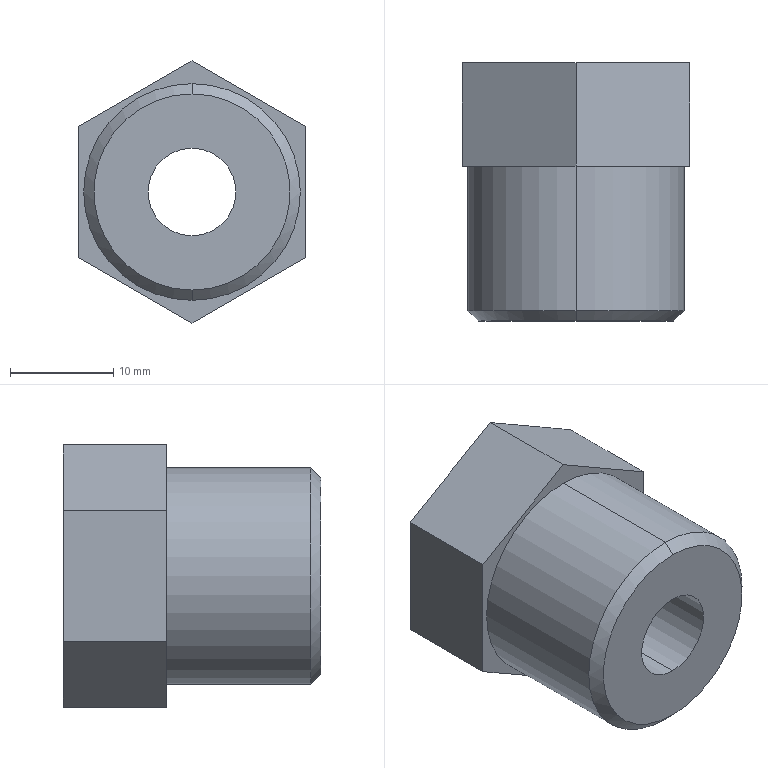Part | SolidWorks | features 3DProfileFeature 1, Chamfer 1, Extrusion 1, HoleWzd 1, ICE 1 | 1 solid | 15 faces | box 22 x 25 x 25.403 mm | volume 7936 mm3 | plane 9 | cylinder 4 | cone 2 | commonest cylinder face diameters 8.5 x2 21 x2
STEP:
#1=CARTESIAN_POINT('',(0.,0.,-4.25));
#2=VERTEX_POINT('',#1);
#3=CARTESIAN_POINT('',(0.,0.,4.25));
#4=VERTEX_POINT('',#3);
#5=CARTESIAN_POINT('',(0.,0.,0.));
#6=DIRECTION('',(0.,1.,0.));
#7=DIRECTION('',(0.,0.,1.));
#8=AXIS2_PLACEMENT_3D('',#5,#6,#7);
#9=CIRCLE('',#8,4.25);
#10=EDGE_CURVE('',#2,#4,#9,.T.);
#11=ORIENTED_EDGE('',*,*,#10,.F.);
#12=CARTESIAN_POINT('',(0.,25.,-4.25));
#13=VERTEX_POINT('',#12);
#14=CARTESIAN_POINT('',(0.,25.,-4.25));
#15=DIRECTION('',(0.,1.,0.));
#16=VECTOR('',#15,1000.);
#17=LINE('',#14,#16);
#18=EDGE_CURVE('',#2,#13,#17,.T.);
#19=ORIENTED_EDGE('',*,*,#18,.T.);
#20=CARTESIAN_POINT('',(0.,25.,4.25));
#21=VERTEX_POINT('',#20);
#22=CARTESIAN_POINT('',(0.,25.,0.));
#23=DIRECTION('',(0.,1.,0.));
#24=DIRECTION('',(0.,0.,1.));
#25=AXIS2_PLACEMENT_3D('',#22,#23,#24);
#26=CIRCLE('',#25,4.25);
#27=EDGE_CURVE('',#13,#21,#26,.T.);
#28=ORIENTED_EDGE('',*,*,#27,.T.);
#29=CARTESIAN_POINT('',(0.,25.,4.25));
#30=DIRECTION('',(0.,1.,0.));
#31=VECTOR('',#30,1000.);
#32=LINE('',#29,#31);
#33=EDGE_CURVE('',#4,#21,#32,.T.);
#34=ORIENTED_EDGE('',*,*,#33,.F.);
#35=EDGE_LOOP('',(#11,#19,#28,#34));
#36=FACE_OUTER_BOUND('',#35,.T.);
#37=CARTESIAN_POINT('',(0.,25.,0.));
#38=DIRECTION('',(0.,1.,0.));
#39=DIRECTION('',(0.,0.,1.));
#40=AXIS2_PLACEMENT_3D('',#37,#38,#39);
#41=CYLINDRICAL_SURFACE('',#40,4.25);
#42=ADVANCED_FACE('',(#36),#41,.F.);
#43=CARTESIAN_POINT('',(0.,0.,-9.5));
#44=VERTEX_POINT('',#43);
#45=CARTESIAN_POINT('',(0.,0.,9.5));
#46=VERTEX_POINT('',#45);
#47=CARTESIAN_POINT('',(0.,0.,0.));
#48=DIRECTION('',(0.,-1.,0.));
#49=DIRECTION('',(0.,0.,1.));
#50=AXIS2_PLACEMENT_3D('',#47,#48,#49);
#51=CIRCLE('',#50,9.5);
#52=EDGE_CURVE('',#44,#46,#51,.T.);
#53=ORIENTED_EDGE('',*,*,#52,.F.);
#54=CARTESIAN_POINT('',(0.,1.,-10.5));
#55=VERTEX_POINT('',#54);
#56=CARTESIAN_POINT('',(0.,0.,-9.5));
#57=DIRECTION('',(0.,0.7071,-0.7071));
#58=VECTOR('',#57,1000.);
#59=LINE('',#56,#58);
#60=EDGE_CURVE('',#44,#55,#59,.T.);
#61=ORIENTED_EDGE('',*,*,#60,.T.);
#62=CARTESIAN_POINT('',(0.,1.,10.5));
#63=VERTEX_POINT('',#62);
#64=CARTESIAN_POINT('',(0.,1.,0.));
#65=DIRECTION('',(0.,1.,0.));
#66=DIRECTION('',(0.,0.,1.));
#67=AXIS2_PLACEMENT_3D('',#64,#65,#66);
#68=CIRCLE('',#67,10.5);
#69=EDGE_CURVE('',#63,#55,#68,.T.);
#70=ORIENTED_EDGE('',*,*,#69,.F.);
#71=CARTESIAN_POINT('',(0.,0.,9.5));
#72=DIRECTION('',(0.,0.7071,0.7071));
#73=VECTOR('',#72,1000.);
#74=LINE('',#71,#73);
#75=EDGE_CURVE('',#46,#63,#74,.T.);
#76=ORIENTED_EDGE('',*,*,#75,.F.);
#77=EDGE_LOOP('',(#53,#61,#70,#76));
#78=FACE_OUTER_BOUND('',#77,.T.);
#79=CARTESIAN_POINT('',(0.,0.,0.));
#80=DIRECTION('',(0.,1.,0.));
#81=DIRECTION('',(0.,0.,1.));
#82=AXIS2_PLACEMENT_3D('',#79,#80,#81);
#83=CONICAL_SURFACE('',#82,9.5,0.7854);
#84=ADVANCED_FACE('',(#78),#83,.T.);
#85=CARTESIAN_POINT('',(0.,15.,-10.5));
#86=VERTEX_POINT('',#85);
#87=CARTESIAN_POINT('',(0.,15.,10.5));
#88=VERTEX_POINT('',#87);
#89=CARTESIAN_POINT('',(0.,15.,0.));
#90=DIRECTION('',(0.,-1.,0.));
#91=DIRECTION('',(0.,0.,1.));
#92=AXIS2_PLACEMENT_3D('',#89,#90,#91);
#93=CIRCLE('',#92,10.5);
#94=EDGE_CURVE('',#86,#88,#93,.T.);
#95=ORIENTED_EDGE('',*,*,#94,.T.);
#96=CARTESIAN_POINT('',(0.,58.942,10.5));
#97=DIRECTION('',(0.,-1.,0.));
#98=VECTOR('',#97,1000.);
#99=LINE('',#96,#98);
#100=EDGE_CURVE('',#88,#63,#99,.T.);
#101=ORIENTED_EDGE('',*,*,#100,.T.);
#102=ORIENTED_EDGE('',*,*,#69,.T.);
#103=CARTESIAN_POINT('',(0.,58.942,-10.5));
#104=DIRECTION('',(0.,-1.,0.));
#105=VECTOR('',#104,1000.);
#106=LINE('',#103,#105);
#107=EDGE_CURVE('',#86,#55,#106,.T.);
#108=ORIENTED_EDGE('',*,*,#107,.F.);
#109=EDGE_LOOP('',(#95,#101,#102,#108));
#110=FACE_OUTER_BOUND('',#109,.T.);
#111=CARTESIAN_POINT('',(0.,58.942,0.));
#112=DIRECTION('',(0.,-1.,0.));
#113=DIRECTION('',(0.,0.,-1.));
#114=AXIS2_PLACEMENT_3D('',#111,#112,#113);
#115=CYLINDRICAL_SURFACE('',#114,10.5);
#116=ADVANCED_FACE('',(#110),#115,.T.);
#117=CARTESIAN_POINT('',(0.,25.,12.702));
#118=VERTEX_POINT('',#117);
#119=CARTESIAN_POINT('',(0.,15.,12.702));
#120=VERTEX_POINT('',#119);
#121=CARTESIAN_POINT('',(0.,25.,12.702));
#122=DIRECTION('',(0.,-1.,0.));
#123=VECTOR('',#122,1000.);
#124=LINE('',#121,#123);
#125=EDGE_CURVE('',#118,#120,#124,.T.);
#126=ORIENTED_EDGE('',*,*,#125,.T.);
#127=CARTESIAN_POINT('',(11.,15.,6.351));
#128=VERTEX_POINT('',#127);
#129=CARTESIAN_POINT('',(0.,15.,12.702));
#130=DIRECTION('',(0.866,0.,-0.5));
#131=VECTOR('',#130,1000.);
#132=LINE('',#129,#131);
#133=EDGE_CURVE('',#120,#128,#132,.T.);
#134=ORIENTED_EDGE('',*,*,#133,.T.);
#135=CARTESIAN_POINT('',(11.,25.,6.351));
#136=VERTEX_POINT('',#135);
#137=CARTESIAN_POINT('',(11.,25.,6.351));
#138=DIRECTION('',(0.,-1.,0.));
#139=VECTOR('',#138,1000.);
#140=LINE('',#137,#139);
#141=EDGE_CURVE('',#136,#128,#140,.T.);
#142=ORIENTED_EDGE('',*,*,#141,.F.);
#143=CARTESIAN_POINT('',(0.,25.,12.702));
#144=DIRECTION('',(0.866,0.,-0.5));
#145=VECTOR('',#144,1000.);
#146=LINE('',#143,#145);
#147=EDGE_CURVE('',#118,#136,#146,.T.);
#148=ORIENTED_EDGE('',*,*,#147,.F.);
#149=EDGE_LOOP('',(#126,#134,#142,#148));
#150=FACE_OUTER_BOUND('',#149,.T.);
#151=CARTESIAN_POINT('',(0.,25.,12.702));
#152=DIRECTION('',(-0.5,0.,-0.866));
#153=DIRECTION('',(-0.866,0.,0.5));
#154=AXIS2_PLACEMENT_3D('',#151,#152,#153);
#155=PLANE('',#154);
#156=ADVANCED_FACE('',(#150),#155,.F.);
#157=ORIENTED_EDGE('',*,*,#141,.T.);
#158=CARTESIAN_POINT('',(11.,15.,-6.351));
#159=VERTEX_POINT('',#158);
#160=CARTESIAN_POINT('',(11.,15.,6.351));
#161=DIRECTION('',(0.,0.,-1.));
#162=VECTOR('',#161,1000.);
#163=LINE('',#160,#162);
#164=EDGE_CURVE('',#128,#159,#163,.T.);
#165=ORIENTED_EDGE('',*,*,#164,.T.);
#166=CARTESIAN_POINT('',(11.,25.,-6.351));
#167=VERTEX_POINT('',#166);
#168=CARTESIAN_POINT('',(11.,25.,-6.351));
#169=DIRECTION('',(0.,-1.,0.));
#170=VECTOR('',#169,1000.);
#171=LINE('',#168,#170);
#172=EDGE_CURVE('',#167,#159,#171,.T.);
#173=ORIENTED_EDGE('',*,*,#172,.F.);
#174=CARTESIAN_POINT('',(11.,25.,6.351));
#175=DIRECTION('',(0.,0.,-1.));
#176=VECTOR('',#175,1000.);
#177=LINE('',#174,#176);
#178=EDGE_CURVE('',#136,#167,#177,.T.);
#179=ORIENTED_EDGE('',*,*,#178,.F.);
#180=EDGE_LOOP('',(#157,#165,#173,#179));
#181=FACE_OUTER_BOUND('',#180,.T.);
#182=CARTESIAN_POINT('',(11.,25.,6.351));
#183=DIRECTION('',(-1.,0.,0.));
#184=DIRECTION('',(0.,0.,1.));
#185=AXIS2_PLACEMENT_3D('',#182,#183,#184);
#186=PLANE('',#185);
#187=ADVANCED_FACE('',(#181),#186,.F.);
#188=ORIENTED_EDGE('',*,*,#172,.T.);
#189=CARTESIAN_POINT('',(0.,15.,-12.702));
#190=VERTEX_POINT('',#189);
#191=CARTESIAN_POINT('',(11.,15.,-6.351));
#192=DIRECTION('',(-0.866,0.,-0.5));
#193=VECTOR('',#192,1000.);
#194=LINE('',#191,#193);
#195=EDGE_CURVE('',#159,#190,#194,.T.);
#196=ORIENTED_EDGE('',*,*,#195,.T.);
#197=CARTESIAN_POINT('',(0.,25.,-12.702));
#198=VERTEX_POINT('',#197);
#199=CARTESIAN_POINT('',(0.,25.,-12.702));
#200=DIRECTION('',(0.,-1.,0.));
#201=VECTOR('',#200,1000.);
#202=LINE('',#199,#201);
#203=EDGE_CURVE('',#198,#190,#202,.T.);
#204=ORIENTED_EDGE('',*,*,#203,.F.);
#205=CARTESIAN_POINT('',(11.,25.,-6.351));
#206=DIRECTION('',(-0.866,0.,-0.5));
#207=VECTOR('',#206,1000.);
#208=LINE('',#205,#207);
#209=EDGE_CURVE('',#167,#198,#208,.T.);
#210=ORIENTED_EDGE('',*,*,#209,.F.);
#211=EDGE_LOOP('',(#188,#196,#204,#210));
#212=FACE_OUTER_BOUND('',#211,.T.);
#213=CARTESIAN_POINT('',(11.,25.,-6.351));
#214=DIRECTION('',(-0.5,0.,0.866));
#215=DIRECTION('',(0.866,0.,0.5));
#216=AXIS2_PLACEMENT_3D('',#213,#214,#215);
#217=PLANE('',#216);
#218=ADVANCED_FACE('',(#212),#217,.F.);
#219=ORIENTED_EDGE('',*,*,#203,.T.);
#220=CARTESIAN_POINT('',(-11.,15.,-6.351));
#221=VERTEX_POINT('',#220);
#222=CARTESIAN_POINT('',(0.,15.,-12.702));
#223=DIRECTION('',(-0.866,0.,0.5));
#224=VECTOR('',#223,1000.);
#225=LINE('',#222,#224);
#226=EDGE_CURVE('',#190,#221,#225,.T.);
#227=ORIENTED_EDGE('',*,*,#226,.T.);
#228=CARTESIAN_POINT('',(-11.,25.,-6.351));
#229=VERTEX_POINT('',#228);
#230=CARTESIAN_POINT('',(-11.,25.,-6.351));
#231=DIRECTION('',(0.,-1.,0.));
#232=VECTOR('',#231,1000.);
#233=LINE('',#230,#232);
#234=EDGE_CURVE('',#229,#221,#233,.T.);
#235=ORIENTED_EDGE('',*,*,#234,.F.);
#236=CARTESIAN_POINT('',(0.,25.,-12.702));
#237=DIRECTION('',(-0.866,0.,0.5));
#238=VECTOR('',#237,1000.);
#239=LINE('',#236,#238);
#240=EDGE_CURVE('',#198,#229,#239,.T.);
#241=ORIENTED_EDGE('',*,*,#240,.F.);
#242=EDGE_LOOP('',(#219,#227,#235,#241));
#243=FACE_OUTER_BOUND('',#242,.T.);
#244=CARTESIAN_POINT('',(0.,25.,-12.702));
#245=DIRECTION('',(0.5,0.,0.866));
#246=DIRECTION('',(0.866,0.,-0.5));
#247=AXIS2_PLACEMENT_3D('',#244,#245,#246);
#248=PLANE('',#247);
#249=ADVANCED_FACE('',(#243),#248,.F.);
#250=ORIENTED_EDGE('',*,*,#234,.T.);
#251=CARTESIAN_POINT('',(-11.,15.,6.351));
#252=VERTEX_POINT('',#251);
#253=CARTESIAN_POINT('',(-11.,15.,-6.351));
#254=DIRECTION('',(0.,0.,1.));
#255=VECTOR('',#254,1000.);
#256=LINE('',#253,#255);
#257=EDGE_CURVE('',#221,#252,#256,.T.);
#258=ORIENTED_EDGE('',*,*,#257,.T.);
#259=CARTESIAN_POINT('',(-11.,25.,6.351));
#260=VERTEX_POINT('',#259);
#261=CARTESIAN_POINT('',(-11.,25.,6.351));
#262=DIRECTION('',(0.,-1.,0.));
#263=VECTOR('',#262,1000.);
#264=LINE('',#261,#263);
#265=EDGE_CURVE('',#260,#252,#264,.T.);
#266=ORIENTED_EDGE('',*,*,#265,.F.);
#267=CARTESIAN_POINT('',(-11.,25.,-6.351));
#268=DIRECTION('',(0.,0.,1.));
#269=VECTOR('',#268,1000.);
#270=LINE('',#267,#269);
#271=EDGE_CURVE('',#229,#260,#270,.T.);
#272=ORIENTED_EDGE('',*,*,#271,.F.);
#273=EDGE_LOOP('',(#250,#258,#266,#272));
#274=FACE_OUTER_BOUND('',#273,.T.);
#275=CARTESIAN_POINT('',(-11.,25.,-6.351));
#276=DIRECTION('',(1.,0.,0.));
#277=DIRECTION('',(0.,0.,-1.));
#278=AXIS2_PLACEMENT_3D('',#275,#276,#277);
#279=PLANE('',#278);
#280=ADVANCED_FACE('',(#274),#279,.F.);
#281=ORIENTED_EDGE('',*,*,#265,.T.);
#282=CARTESIAN_POINT('',(-11.,15.,6.351));
#283=DIRECTION('',(0.866,0.,0.5));
#284=VECTOR('',#283,1000.);
#285=LINE('',#282,#284);
#286=EDGE_CURVE('',#252,#120,#285,.T.);
#287=ORIENTED_EDGE('',*,*,#286,.T.);
#288=ORIENTED_EDGE('',*,*,#125,.F.);
#289=CARTESIAN_POINT('',(-11.,25.,6.351));
#290=DIRECTION('',(0.866,0.,0.5));
#291=VECTOR('',#290,1000.);
#292=LINE('',#289,#291);
#293=EDGE_CURVE('',#260,#118,#292,.T.);
#294=ORIENTED_EDGE('',*,*,#293,.F.);
#295=EDGE_LOOP('',(#281,#287,#288,#294));
#296=FACE_OUTER_BOUND('',#295,.T.);
#297=CARTESIAN_POINT('',(-11.,25.,6.351));
#298=DIRECTION('',(0.5,0.,-0.866));
#299=DIRECTION('',(-0.866,0.,-0.5));
#300=AXIS2_PLACEMENT_3D('',#297,#298,#299);
#301=PLANE('',#300);
#302=ADVANCED_FACE('',(#296),#301,.F.);
#303=CARTESIAN_POINT('',(0.,25.,0.));
#304=DIRECTION('',(0.,1.,0.));
#305=DIRECTION('',(0.,0.,1.));
#306=AXIS2_PLACEMENT_3D('',#303,#304,#305);
#307=CIRCLE('',#306,4.25);
#308=EDGE_CURVE('',#21,#13,#307,.T.);
#309=ORIENTED_EDGE('',*,*,#308,.F.);
#310=ORIENTED_EDGE('',*,*,#27,.F.);
#311=EDGE_LOOP('',(#309,#310));
#312=FACE_BOUND('',#311,.T.);
#313=ORIENTED_EDGE('',*,*,#147,.T.);
#314=ORIENTED_EDGE('',*,*,#178,.T.);
#315=ORIENTED_EDGE('',*,*,#209,.T.);
#316=ORIENTED_EDGE('',*,*,#240,.T.);
#317=ORIENTED_EDGE('',*,*,#271,.T.);
#318=ORIENTED_EDGE('',*,*,#293,.T.);
#319=EDGE_LOOP('',(#313,#314,#315,#316,#317,#318));
#320=FACE_OUTER_BOUND('',#319,.T.);
#321=CARTESIAN_POINT('',(0.,25.,0.));
#322=DIRECTION('',(0.,1.,0.));
#323=DIRECTION('',(0.,0.,1.));
#324=AXIS2_PLACEMENT_3D('',#321,#322,#323);
#325=PLANE('',#324);
#326=ADVANCED_FACE('',(#312,#320),#325,.T.);
#327=ORIENTED_EDGE('',*,*,#94,.F.);
#328=CARTESIAN_POINT('',(0.,15.,0.));
#329=DIRECTION('',(0.,-1.,0.));
#330=DIRECTION('',(0.,0.,1.));
#331=AXIS2_PLACEMENT_3D('',#328,#329,#330);
#332=CIRCLE('',#331,10.5);
#333=EDGE_CURVE('',#88,#86,#332,.T.);
#334=ORIENTED_EDGE('',*,*,#333,.F.);
#335=EDGE_LOOP('',(#327,#334));
#336=FACE_BOUND('',#335,.T.);
#337=ORIENTED_EDGE('',*,*,#286,.F.);
#338=ORIENTED_EDGE('',*,*,#257,.F.);
#339=ORIENTED_EDGE('',*,*,#226,.F.);
#340=ORIENTED_EDGE('',*,*,#195,.F.);
#341=ORIENTED_EDGE('',*,*,#164,.F.);
#342=ORIENTED_EDGE('',*,*,#133,.F.);
#343=EDGE_LOOP('',(#337,#338,#339,#340,#341,#342));
#344=FACE_OUTER_BOUND('',#343,.T.);
#345=CARTESIAN_POINT('',(0.,15.,0.));
#346=DIRECTION('',(0.,1.,0.));
#347=DIRECTION('',(0.,0.,1.));
#348=AXIS2_PLACEMENT_3D('',#345,#346,#347);
#349=PLANE('',#348);
#350=ADVANCED_FACE('',(#336,#344),#349,.F.);
#351=ORIENTED_EDGE('',*,*,#100,.F.);
#352=ORIENTED_EDGE('',*,*,#333,.T.);
#353=ORIENTED_EDGE('',*,*,#107,.T.);
#354=CARTESIAN_POINT('',(0.,1.,0.));
#355=DIRECTION('',(0.,1.,0.));
#356=DIRECTION('',(0.,0.,1.));
#357=AXIS2_PLACEMENT_3D('',#354,#355,#356);
#358=CIRCLE('',#357,10.5);
#359=EDGE_CURVE('',#55,#63,#358,.T.);
#360=ORIENTED_EDGE('',*,*,#359,.T.);
#361=EDGE_LOOP('',(#351,#352,#353,#360));
#362=FACE_OUTER_BOUND('',#361,.T.);
#363=CARTESIAN_POINT('',(0.,58.942,0.));
#364=DIRECTION('',(0.,-1.,0.));
#365=DIRECTION('',(0.,0.,-1.));
#366=AXIS2_PLACEMENT_3D('',#363,#364,#365);
#367=CYLINDRICAL_SURFACE('',#366,10.5);
#368=ADVANCED_FACE('',(#362),#367,.T.);
#369=CARTESIAN_POINT('',(0.,0.,0.));
#370=DIRECTION('',(0.,1.,0.));
#371=DIRECTION('',(0.,0.,1.));
#372=AXIS2_PLACEMENT_3D('',#369,#370,#371);
#373=CIRCLE('',#372,4.25);
#374=EDGE_CURVE('',#4,#2,#373,.T.);
#375=ORIENTED_EDGE('',*,*,#374,.T.);
#376=ORIENTED_EDGE('',*,*,#10,.T.);
#377=EDGE_LOOP('',(#375,#376));
#378=FACE_BOUND('',#377,.T.);
#379=CARTESIAN_POINT('',(0.,0.,0.));
#380=DIRECTION('',(0.,-1.,0.));
#381=DIRECTION('',(0.,0.,1.));
#382=AXIS2_PLACEMENT_3D('',#379,#380,#381);
#383=CIRCLE('',#382,9.5);
#384=EDGE_CURVE('',#46,#44,#383,.T.);
#385=ORIENTED_EDGE('',*,*,#384,.T.);
#386=ORIENTED_EDGE('',*,*,#52,.T.);
#387=EDGE_LOOP('',(#385,#386));
#388=FACE_OUTER_BOUND('',#387,.T.);
#389=CARTESIAN_POINT('',(0.,0.,0.));
#390=DIRECTION('',(0.,1.,0.));
#391=DIRECTION('',(0.,0.,1.));
#392=AXIS2_PLACEMENT_3D('',#389,#390,#391);
#393=PLANE('',#392);
#394=ADVANCED_FACE('',(#378,#388),#393,.F.);
#395=ORIENTED_EDGE('',*,*,#60,.F.);
#396=ORIENTED_EDGE('',*,*,#384,.F.);
#397=ORIENTED_EDGE('',*,*,#75,.T.);
#398=ORIENTED_EDGE('',*,*,#359,.F.);
#399=EDGE_LOOP('',(#395,#396,#397,#398));
#400=FACE_OUTER_BOUND('',#399,.T.);
#401=CARTESIAN_POINT('',(0.,0.,0.));
#402=DIRECTION('',(0.,1.,0.));
#403=DIRECTION('',(0.,0.,1.));
#404=AXIS2_PLACEMENT_3D('',#401,#402,#403);
#405=CONICAL_SURFACE('',#404,9.5,0.7854);
#406=ADVANCED_FACE('',(#400),#405,.T.);
#407=ORIENTED_EDGE('',*,*,#18,.F.);
#408=ORIENTED_EDGE('',*,*,#374,.F.);
#409=ORIENTED_EDGE('',*,*,#33,.T.);
#410=ORIENTED_EDGE('',*,*,#308,.T.);
#411=EDGE_LOOP('',(#407,#408,#409,#410));
#412=FACE_OUTER_BOUND('',#411,.T.);
#413=CARTESIAN_POINT('',(0.,25.,0.));
#414=DIRECTION('',(0.,1.,0.));
#415=DIRECTION('',(0.,0.,1.));
#416=AXIS2_PLACEMENT_3D('',#413,#414,#415);
#417=CYLINDRICAL_SURFACE('',#416,4.25);
#418=ADVANCED_FACE('',(#412),#417,.F.);
#419=CLOSED_SHELL('',(#42,#84,#116,#156,#187,#218,#249,#280,#302,#326,#350,#368,#394,#406,#418));
#420=MANIFOLD_SOLID_BREP('',#419);
#421=CARTESIAN_POINT('',(0.,0.,0.));
#422=DIRECTION('',(0.,0.,1.));
#423=DIRECTION('',(1.,0.,0.));
#424=AXIS2_PLACEMENT_3D('',#421,#422,#423);
#425=(LENGTH_UNIT()NAMED_UNIT(*)SI_UNIT(.MILLI.,.METRE.));
#426=UNCERTAINTY_MEASURE_WITH_UNIT(LENGTH_MEASURE(0.00001),#425,'','');
#427=(NAMED_UNIT(*)PLANE_ANGLE_UNIT()SI_UNIT($,.RADIAN.));
#428=(NAMED_UNIT(*)SI_UNIT($,.STERADIAN.)SOLID_ANGLE_UNIT());
#429=(GEOMETRIC_REPRESENTATION_CONTEXT(3)GLOBAL_UNCERTAINTY_ASSIGNED_CONTEXT((#426))GLOBAL_UNIT_ASSIGNED_CONTEXT((#425,#427,#428))REPRESENTATION_CONTEXT('',''));
#430=ADVANCED_BREP_SHAPE_REPRESENTATION('',(#420,#424),#429);